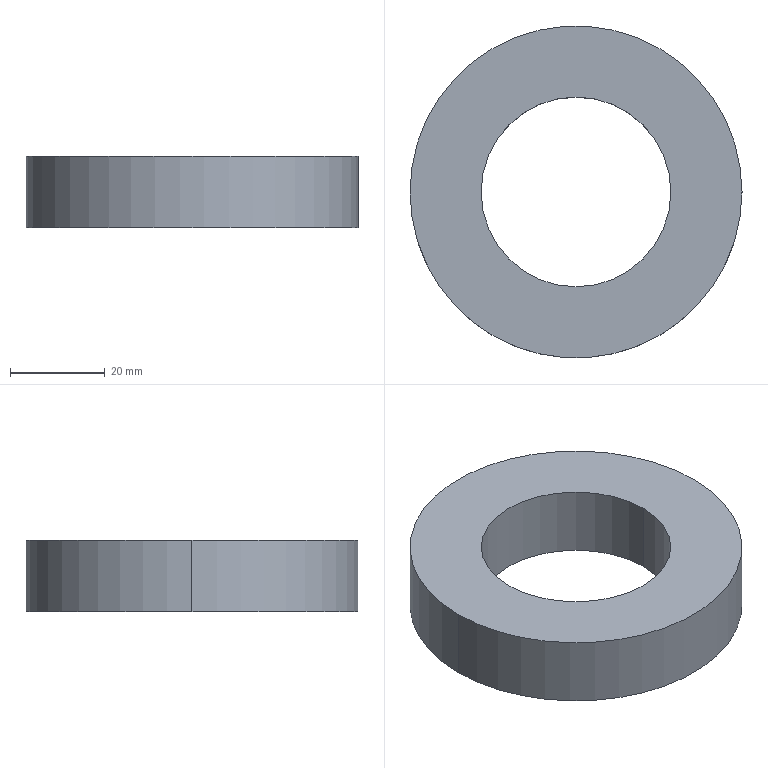Part | SolidWorks | features Extrusion 1 | 1 solid | 6 faces | box 70 x 70 x 15 mm | volume 38877 mm3 | cylinder 4 | plane 2 | commonest cylinder face diameters 40 x2 70 x2
STEP:
#1=CARTESIAN_POINT('',(-20.,0.,15.));
#2=VERTEX_POINT('',#1);
#3=CARTESIAN_POINT('',(20.,0.,15.));
#4=VERTEX_POINT('',#3);
#5=CARTESIAN_POINT('',(0.,0.,15.));
#6=DIRECTION('',(0.,0.,1.));
#7=DIRECTION('',(1.,0.,0.));
#8=AXIS2_PLACEMENT_3D('',#5,#6,#7);
#9=CIRCLE('',#8,20.);
#10=EDGE_CURVE('',#2,#4,#9,.T.);
#11=ORIENTED_EDGE('',*,*,#10,.T.);
#12=CARTESIAN_POINT('',(20.,0.,0.));
#13=VERTEX_POINT('',#12);
#14=CARTESIAN_POINT('',(20.,0.,15.));
#15=DIRECTION('',(0.,0.,-1.));
#16=VECTOR('',#15,1000.);
#17=LINE('',#14,#16);
#18=EDGE_CURVE('',#4,#13,#17,.T.);
#19=ORIENTED_EDGE('',*,*,#18,.T.);
#20=CARTESIAN_POINT('',(-20.,0.,0.));
#21=VERTEX_POINT('',#20);
#22=CARTESIAN_POINT('',(0.,0.,0.));
#23=DIRECTION('',(0.,0.,1.));
#24=DIRECTION('',(1.,0.,0.));
#25=AXIS2_PLACEMENT_3D('',#22,#23,#24);
#26=CIRCLE('',#25,20.);
#27=EDGE_CURVE('',#21,#13,#26,.T.);
#28=ORIENTED_EDGE('',*,*,#27,.F.);
#29=CARTESIAN_POINT('',(-20.,0.,15.));
#30=DIRECTION('',(0.,0.,-1.));
#31=VECTOR('',#30,1000.);
#32=LINE('',#29,#31);
#33=EDGE_CURVE('',#2,#21,#32,.T.);
#34=ORIENTED_EDGE('',*,*,#33,.F.);
#35=EDGE_LOOP('',(#11,#19,#28,#34));
#36=FACE_OUTER_BOUND('',#35,.T.);
#37=CARTESIAN_POINT('',(0.,0.,15.));
#38=DIRECTION('',(0.,0.,-1.));
#39=DIRECTION('',(-1.,0.,0.));
#40=AXIS2_PLACEMENT_3D('',#37,#38,#39);
#41=CYLINDRICAL_SURFACE('',#40,20.);
#42=ADVANCED_FACE('',(#36),#41,.F.);
#43=CARTESIAN_POINT('',(35.,0.,15.));
#44=VERTEX_POINT('',#43);
#45=CARTESIAN_POINT('',(-35.,0.,15.));
#46=VERTEX_POINT('',#45);
#47=CARTESIAN_POINT('',(0.,0.,15.));
#48=DIRECTION('',(0.,0.,1.));
#49=DIRECTION('',(1.,0.,0.));
#50=AXIS2_PLACEMENT_3D('',#47,#48,#49);
#51=CIRCLE('',#50,35.);
#52=EDGE_CURVE('',#44,#46,#51,.T.);
#53=ORIENTED_EDGE('',*,*,#52,.F.);
#54=CARTESIAN_POINT('',(35.,0.,0.));
#55=VERTEX_POINT('',#54);
#56=CARTESIAN_POINT('',(35.,0.,15.));
#57=DIRECTION('',(0.,0.,-1.));
#58=VECTOR('',#57,1000.);
#59=LINE('',#56,#58);
#60=EDGE_CURVE('',#44,#55,#59,.T.);
#61=ORIENTED_EDGE('',*,*,#60,.T.);
#62=CARTESIAN_POINT('',(-35.,0.,0.));
#63=VERTEX_POINT('',#62);
#64=CARTESIAN_POINT('',(0.,0.,0.));
#65=DIRECTION('',(0.,0.,1.));
#66=DIRECTION('',(1.,0.,0.));
#67=AXIS2_PLACEMENT_3D('',#64,#65,#66);
#68=CIRCLE('',#67,35.);
#69=EDGE_CURVE('',#55,#63,#68,.T.);
#70=ORIENTED_EDGE('',*,*,#69,.T.);
#71=CARTESIAN_POINT('',(-35.,0.,15.));
#72=DIRECTION('',(0.,0.,-1.));
#73=VECTOR('',#72,1000.);
#74=LINE('',#71,#73);
#75=EDGE_CURVE('',#46,#63,#74,.T.);
#76=ORIENTED_EDGE('',*,*,#75,.F.);
#77=EDGE_LOOP('',(#53,#61,#70,#76));
#78=FACE_OUTER_BOUND('',#77,.T.);
#79=CARTESIAN_POINT('',(0.,0.,15.));
#80=DIRECTION('',(0.,0.,-1.));
#81=DIRECTION('',(-1.,0.,0.));
#82=AXIS2_PLACEMENT_3D('',#79,#80,#81);
#83=CYLINDRICAL_SURFACE('',#82,35.);
#84=ADVANCED_FACE('',(#78),#83,.T.);
#85=CARTESIAN_POINT('',(0.,0.,15.));
#86=DIRECTION('',(0.,0.,1.));
#87=DIRECTION('',(1.,0.,0.));
#88=AXIS2_PLACEMENT_3D('',#85,#86,#87);
#89=CIRCLE('',#88,35.);
#90=EDGE_CURVE('',#46,#44,#89,.T.);
#91=ORIENTED_EDGE('',*,*,#90,.T.);
#92=ORIENTED_EDGE('',*,*,#52,.T.);
#93=EDGE_LOOP('',(#91,#92));
#94=FACE_OUTER_BOUND('',#93,.T.);
#95=ORIENTED_EDGE('',*,*,#10,.F.);
#96=CARTESIAN_POINT('',(0.,0.,15.));
#97=DIRECTION('',(0.,0.,1.));
#98=DIRECTION('',(1.,0.,0.));
#99=AXIS2_PLACEMENT_3D('',#96,#97,#98);
#100=CIRCLE('',#99,20.);
#101=EDGE_CURVE('',#4,#2,#100,.T.);
#102=ORIENTED_EDGE('',*,*,#101,.F.);
#103=EDGE_LOOP('',(#95,#102));
#104=FACE_BOUND('',#103,.T.);
#105=CARTESIAN_POINT('',(0.,0.,15.));
#106=DIRECTION('',(0.,0.,1.));
#107=DIRECTION('',(1.,0.,0.));
#108=AXIS2_PLACEMENT_3D('',#105,#106,#107);
#109=PLANE('',#108);
#110=ADVANCED_FACE('',(#94,#104),#109,.T.);
#111=CARTESIAN_POINT('',(0.,0.,0.));
#112=DIRECTION('',(0.,0.,1.));
#113=DIRECTION('',(1.,0.,0.));
#114=AXIS2_PLACEMENT_3D('',#111,#112,#113);
#115=CIRCLE('',#114,35.);
#116=EDGE_CURVE('',#63,#55,#115,.T.);
#117=ORIENTED_EDGE('',*,*,#116,.F.);
#118=ORIENTED_EDGE('',*,*,#69,.F.);
#119=EDGE_LOOP('',(#117,#118));
#120=FACE_OUTER_BOUND('',#119,.T.);
#121=ORIENTED_EDGE('',*,*,#27,.T.);
#122=CARTESIAN_POINT('',(0.,0.,0.));
#123=DIRECTION('',(0.,0.,1.));
#124=DIRECTION('',(1.,0.,0.));
#125=AXIS2_PLACEMENT_3D('',#122,#123,#124);
#126=CIRCLE('',#125,20.);
#127=EDGE_CURVE('',#13,#21,#126,.T.);
#128=ORIENTED_EDGE('',*,*,#127,.T.);
#129=EDGE_LOOP('',(#121,#128));
#130=FACE_BOUND('',#129,.T.);
#131=CARTESIAN_POINT('',(0.,0.,0.));
#132=DIRECTION('',(0.,0.,1.));
#133=DIRECTION('',(1.,0.,0.));
#134=AXIS2_PLACEMENT_3D('',#131,#132,#133);
#135=PLANE('',#134);
#136=ADVANCED_FACE('',(#120,#130),#135,.F.);
#137=ORIENTED_EDGE('',*,*,#60,.F.);
#138=ORIENTED_EDGE('',*,*,#90,.F.);
#139=ORIENTED_EDGE('',*,*,#75,.T.);
#140=ORIENTED_EDGE('',*,*,#116,.T.);
#141=EDGE_LOOP('',(#137,#138,#139,#140));
#142=FACE_OUTER_BOUND('',#141,.T.);
#143=CARTESIAN_POINT('',(0.,0.,15.));
#144=DIRECTION('',(0.,0.,-1.));
#145=DIRECTION('',(-1.,0.,0.));
#146=AXIS2_PLACEMENT_3D('',#143,#144,#145);
#147=CYLINDRICAL_SURFACE('',#146,35.);
#148=ADVANCED_FACE('',(#142),#147,.T.);
#149=ORIENTED_EDGE('',*,*,#18,.F.);
#150=ORIENTED_EDGE('',*,*,#101,.T.);
#151=ORIENTED_EDGE('',*,*,#33,.T.);
#152=ORIENTED_EDGE('',*,*,#127,.F.);
#153=EDGE_LOOP('',(#149,#150,#151,#152));
#154=FACE_OUTER_BOUND('',#153,.T.);
#155=CARTESIAN_POINT('',(0.,0.,15.));
#156=DIRECTION('',(0.,0.,-1.));
#157=DIRECTION('',(-1.,0.,0.));
#158=AXIS2_PLACEMENT_3D('',#155,#156,#157);
#159=CYLINDRICAL_SURFACE('',#158,20.);
#160=ADVANCED_FACE('',(#154),#159,.F.);
#161=CLOSED_SHELL('',(#42,#84,#110,#136,#148,#160));
#162=MANIFOLD_SOLID_BREP('',#161);
#163=CARTESIAN_POINT('',(0.,0.,0.));
#164=DIRECTION('',(0.,0.,1.));
#165=DIRECTION('',(1.,0.,0.));
#166=AXIS2_PLACEMENT_3D('',#163,#164,#165);
#167=(LENGTH_UNIT()NAMED_UNIT(*)SI_UNIT(.MILLI.,.METRE.));
#168=UNCERTAINTY_MEASURE_WITH_UNIT(LENGTH_MEASURE(0.00001),#167,'','');
#169=(NAMED_UNIT(*)PLANE_ANGLE_UNIT()SI_UNIT($,.RADIAN.));
#170=(NAMED_UNIT(*)SI_UNIT($,.STERADIAN.)SOLID_ANGLE_UNIT());
#171=(GEOMETRIC_REPRESENTATION_CONTEXT(3)GLOBAL_UNCERTAINTY_ASSIGNED_CONTEXT((#168))GLOBAL_UNIT_ASSIGNED_CONTEXT((#167,#169,#170))REPRESENTATION_CONTEXT('',''));
#172=ADVANCED_BREP_SHAPE_REPRESENTATION('',(#162,#166),#171);